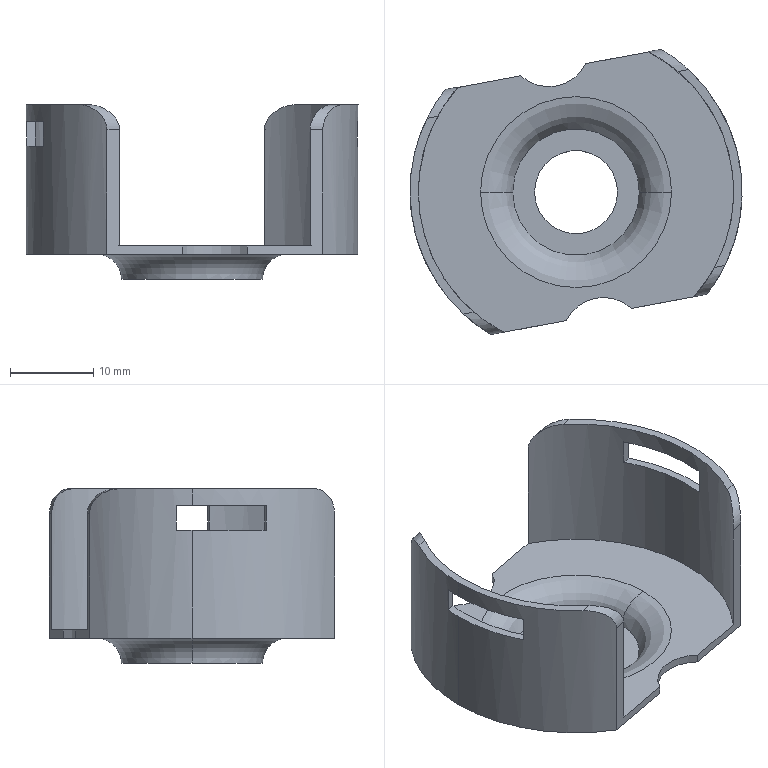Part | SolidWorks | features Cut 4, Fillet 2, Extrusion 1, ICE 1, Shell 1 | 1 solid | 36 faces | box 40 x 34.338 x 21 mm | volume 2143 mm3 | plane 18 | cylinder 14 | torus 4 | commonest cylinder face diameters 6 x4 10 x4 38 x3 40 x3
STEP:
#1=CARTESIAN_POINT('',(-126.531,115.619,0.));
#2=VERTEX_POINT('',#1);
#3=CARTESIAN_POINT('',(-116.531,115.619,0.));
#4=VERTEX_POINT('',#3);
#5=CARTESIAN_POINT('',(-121.531,115.619,0.));
#6=DIRECTION('',(0.,0.,1.));
#7=DIRECTION('',(1.,0.,0.));
#8=AXIS2_PLACEMENT_3D('',#5,#6,#7);
#9=CIRCLE('',#8,5.);
#10=EDGE_CURVE('',#2,#4,#9,.T.);
#11=ORIENTED_EDGE('',*,*,#10,.F.);
#12=CARTESIAN_POINT('',(-126.531,115.619,1.));
#13=VERTEX_POINT('',#12);
#14=CARTESIAN_POINT('',(-126.531,115.619,0.));
#15=DIRECTION('',(0.,0.,1.));
#16=VECTOR('',#15,1000.);
#17=LINE('',#14,#16);
#18=EDGE_CURVE('',#2,#13,#17,.T.);
#19=ORIENTED_EDGE('',*,*,#18,.T.);
#20=CARTESIAN_POINT('',(-116.531,115.619,1.));
#21=VERTEX_POINT('',#20);
#22=CARTESIAN_POINT('',(-121.531,115.619,1.));
#23=DIRECTION('',(0.,0.,-1.));
#24=DIRECTION('',(-1.,0.,0.));
#25=AXIS2_PLACEMENT_3D('',#22,#23,#24);
#26=CIRCLE('',#25,5.);
#27=EDGE_CURVE('',#21,#13,#26,.T.);
#28=ORIENTED_EDGE('',*,*,#27,.F.);
#29=CARTESIAN_POINT('',(-116.531,115.619,0.));
#30=DIRECTION('',(0.,0.,1.));
#31=VECTOR('',#30,1000.);
#32=LINE('',#29,#31);
#33=EDGE_CURVE('',#4,#21,#32,.T.);
#34=ORIENTED_EDGE('',*,*,#33,.F.);
#35=EDGE_LOOP('',(#11,#19,#28,#34));
#36=FACE_OUTER_BOUND('',#35,.T.);
#37=CARTESIAN_POINT('',(-121.531,115.619,0.));
#38=DIRECTION('',(0.,0.,1.));
#39=DIRECTION('',(1.,0.,0.));
#40=AXIS2_PLACEMENT_3D('',#37,#38,#39);
#41=CYLINDRICAL_SURFACE('',#40,5.);
#42=ADVANCED_FACE('',(#36),#41,.F.);
#43=CARTESIAN_POINT('',(-110.031,115.619,4.));
#44=VERTEX_POINT('',#43);
#45=CARTESIAN_POINT('',(-133.031,115.619,4.));
#46=VERTEX_POINT('',#45);
#47=CARTESIAN_POINT('',(-121.531,115.619,4.));
#48=DIRECTION('',(0.,0.,1.));
#49=DIRECTION('',(1.,0.,0.));
#50=AXIS2_PLACEMENT_3D('',#47,#48,#49);
#51=CIRCLE('',#50,11.5);
#52=EDGE_CURVE('',#44,#46,#51,.T.);
#53=ORIENTED_EDGE('',*,*,#52,.T.);
#54=CARTESIAN_POINT('',(-129.158,115.619,1.));
#55=VERTEX_POINT('',#54);
#56=CARTESIAN_POINT('',(-133.031,115.619,0.));
#57=DIRECTION('',(0.,1.,0.));
#58=DIRECTION('',(-1.,0.,0.));
#59=AXIS2_PLACEMENT_3D('',#56,#57,#58);
#60=CIRCLE('',#59,4.);
#61=EDGE_CURVE('',#46,#55,#60,.T.);
#62=ORIENTED_EDGE('',*,*,#61,.T.);
#63=CARTESIAN_POINT('',(-113.904,115.619,1.));
#64=VERTEX_POINT('',#63);
#65=CARTESIAN_POINT('',(-121.531,115.619,1.));
#66=DIRECTION('',(0.,0.,-1.));
#67=DIRECTION('',(1.,0.,0.));
#68=AXIS2_PLACEMENT_3D('',#65,#66,#67);
#69=CIRCLE('',#68,7.627);
#70=EDGE_CURVE('',#55,#64,#69,.T.);
#71=ORIENTED_EDGE('',*,*,#70,.T.);
#72=CARTESIAN_POINT('',(-110.031,115.619,0.));
#73=DIRECTION('',(0.,-1.,0.));
#74=DIRECTION('',(0.,0.,-1.));
#75=AXIS2_PLACEMENT_3D('',#72,#73,#74);
#76=CIRCLE('',#75,4.);
#77=EDGE_CURVE('',#44,#64,#76,.T.);
#78=ORIENTED_EDGE('',*,*,#77,.F.);
#79=EDGE_LOOP('',(#53,#62,#71,#78));
#80=FACE_OUTER_BOUND('',#79,.T.);
#81=CARTESIAN_POINT('',(-121.531,115.619,0.));
#82=DIRECTION('',(0.,0.,1.));
#83=DIRECTION('',(1.,0.,0.));
#84=AXIS2_PLACEMENT_3D('',#81,#82,#83);
#85=TOROIDAL_SURFACE('',#84,11.5,4.);
#86=ADVANCED_FACE('',(#80),#85,.T.);
#87=CARTESIAN_POINT('',(-133.031,115.619,3.));
#88=VERTEX_POINT('',#87);
#89=CARTESIAN_POINT('',(-110.031,115.619,3.));
#90=VERTEX_POINT('',#89);
#91=CARTESIAN_POINT('',(-121.531,115.619,3.));
#92=DIRECTION('',(0.,0.,1.));
#93=DIRECTION('',(1.,0.,0.));
#94=AXIS2_PLACEMENT_3D('',#91,#92,#93);
#95=CIRCLE('',#94,11.5);
#96=EDGE_CURVE('',#88,#90,#95,.T.);
#97=ORIENTED_EDGE('',*,*,#96,.F.);
#98=CARTESIAN_POINT('',(-130.031,115.619,0.));
#99=VERTEX_POINT('',#98);
#100=CARTESIAN_POINT('',(-133.031,115.619,0.));
#101=DIRECTION('',(0.,1.,0.));
#102=DIRECTION('',(-1.,0.,0.));
#103=AXIS2_PLACEMENT_3D('',#100,#101,#102);
#104=CIRCLE('',#103,3.);
#105=EDGE_CURVE('',#88,#99,#104,.T.);
#106=ORIENTED_EDGE('',*,*,#105,.T.);
#107=CARTESIAN_POINT('',(-113.031,115.619,0.));
#108=VERTEX_POINT('',#107);
#109=CARTESIAN_POINT('',(-121.531,115.619,0.));
#110=DIRECTION('',(0.,0.,-1.));
#111=DIRECTION('',(-1.,0.,0.));
#112=AXIS2_PLACEMENT_3D('',#109,#110,#111);
#113=CIRCLE('',#112,8.5);
#114=EDGE_CURVE('',#108,#99,#113,.T.);
#115=ORIENTED_EDGE('',*,*,#114,.F.);
#116=CARTESIAN_POINT('',(-110.031,115.619,0.));
#117=DIRECTION('',(0.,-1.,0.));
#118=DIRECTION('',(0.,0.,-1.));
#119=AXIS2_PLACEMENT_3D('',#116,#117,#118);
#120=CIRCLE('',#119,3.);
#121=EDGE_CURVE('',#90,#108,#120,.T.);
#122=ORIENTED_EDGE('',*,*,#121,.F.);
#123=EDGE_LOOP('',(#97,#106,#115,#122));
#124=FACE_OUTER_BOUND('',#123,.T.);
#125=CARTESIAN_POINT('',(-121.531,115.619,0.));
#126=DIRECTION('',(0.,0.,1.));
#127=DIRECTION('',(1.,0.,0.));
#128=AXIS2_PLACEMENT_3D('',#125,#126,#127);
#129=TOROIDAL_SURFACE('',#128,11.5,3.);
#130=ADVANCED_FACE('',(#124),#129,.F.);
#131=CARTESIAN_POINT('',(-138.211,124.718,21.));
#132=VERTEX_POINT('',#131);
#133=CARTESIAN_POINT('',(-140.531,115.619,21.));
#134=VERTEX_POINT('',#133);
#135=CARTESIAN_POINT('',(-121.531,115.619,21.));
#136=DIRECTION('',(0.,0.,1.));
#137=DIRECTION('',(1.,0.,0.));
#138=AXIS2_PLACEMENT_3D('',#135,#136,#137);
#139=CIRCLE('',#138,19.);
#140=EDGE_CURVE('',#132,#134,#139,.T.);
#141=ORIENTED_EDGE('',*,*,#140,.T.);
#142=CARTESIAN_POINT('',(-140.531,115.619,19.));
#143=VERTEX_POINT('',#142);
#144=CARTESIAN_POINT('',(-140.531,115.619,21.));
#145=DIRECTION('',(0.,0.,-1.));
#146=VECTOR('',#145,1000.);
#147=LINE('',#144,#146);
#148=EDGE_CURVE('',#134,#143,#147,.T.);
#149=ORIENTED_EDGE('',*,*,#148,.T.);
#150=CARTESIAN_POINT('',(-140.417,117.695,19.));
#151=VERTEX_POINT('',#150);
#152=CARTESIAN_POINT('',(-121.531,115.619,19.));
#153=DIRECTION('',(0.,0.,1.));
#154=DIRECTION('',(1.,0.,0.));
#155=AXIS2_PLACEMENT_3D('',#152,#153,#154);
#156=CIRCLE('',#155,19.);
#157=EDGE_CURVE('',#151,#143,#156,.T.);
#158=ORIENTED_EDGE('',*,*,#157,.F.);
#159=CARTESIAN_POINT('',(-140.417,117.695,16.));
#160=VERTEX_POINT('',#159);
#161=CARTESIAN_POINT('',(-140.417,117.695,21.));
#162=DIRECTION('',(0.,0.,1.));
#163=VECTOR('',#162,1000.);
#164=LINE('',#161,#163);
#165=EDGE_CURVE('',#160,#151,#164,.T.);
#166=ORIENTED_EDGE('',*,*,#165,.F.);
#167=CARTESIAN_POINT('',(-140.531,115.619,16.));
#168=VERTEX_POINT('',#167);
#169=CARTESIAN_POINT('',(-121.531,115.619,16.));
#170=DIRECTION('',(0.,0.,-1.));
#171=DIRECTION('',(-1.,0.,0.));
#172=AXIS2_PLACEMENT_3D('',#169,#170,#171);
#173=CIRCLE('',#172,19.);
#174=EDGE_CURVE('',#168,#160,#173,.T.);
#175=ORIENTED_EDGE('',*,*,#174,.F.);
#176=CARTESIAN_POINT('',(-140.531,115.619,4.));
#177=VERTEX_POINT('',#176);
#178=CARTESIAN_POINT('',(-140.531,115.619,21.));
#179=DIRECTION('',(0.,0.,-1.));
#180=VECTOR('',#179,1000.);
#181=LINE('',#178,#180);
#182=EDGE_CURVE('',#168,#177,#181,.T.);
#183=ORIENTED_EDGE('',*,*,#182,.T.);
#184=CARTESIAN_POINT('',(-135.743,128.229,4.));
#185=VERTEX_POINT('',#184);
#186=CARTESIAN_POINT('',(-121.531,115.619,4.));
#187=DIRECTION('',(0.,0.,1.));
#188=DIRECTION('',(1.,0.,0.));
#189=AXIS2_PLACEMENT_3D('',#186,#187,#188);
#190=CIRCLE('',#189,19.);
#191=EDGE_CURVE('',#185,#177,#190,.T.);
#192=ORIENTED_EDGE('',*,*,#191,.F.);
#193=CARTESIAN_POINT('',(-135.743,128.229,18.));
#194=VERTEX_POINT('',#193);
#195=CARTESIAN_POINT('',(-135.743,128.229,21.));
#196=DIRECTION('',(0.,0.,-1.));
#197=VECTOR('',#196,1000.);
#198=LINE('',#195,#197);
#199=EDGE_CURVE('',#194,#185,#198,.T.);
#200=ORIENTED_EDGE('',*,*,#199,.F.);
#201=CARTESIAN_POINT('',(-135.743,128.229,18.));
#202=CARTESIAN_POINT('',(-135.743,128.229,18.243));
#203=CARTESIAN_POINT('',(-135.775,128.194,18.475));
#204=CARTESIAN_POINT('',(-135.889,128.063,18.925));
#205=CARTESIAN_POINT('',(-135.97,127.97,19.132));
#206=CARTESIAN_POINT('',(-136.16,127.745,19.512));
#207=CARTESIAN_POINT('',(-136.267,127.614,19.683));
#208=CARTESIAN_POINT('',(-136.494,127.33,19.99));
#209=CARTESIAN_POINT('',(-136.615,127.174,20.128));
#210=CARTESIAN_POINT('',(-136.984,126.681,20.496));
#211=CARTESIAN_POINT('',(-137.236,126.323,20.678));
#212=CARTESIAN_POINT('',(-137.612,125.741,20.869));
#213=CARTESIAN_POINT('',(-137.736,125.542,20.917));
#214=CARTESIAN_POINT('',(-137.978,125.136,20.983));
#215=CARTESIAN_POINT('',(-138.096,124.929,21.));
#216=CARTESIAN_POINT('',(-138.211,124.718,21.));
#217=B_SPLINE_CURVE_WITH_KNOTS('',3,(#201,#202,#203,#204,#205,#206,#207,#208,#209,#210,#211,#212,#213,#214,#215,#216),.UNSPECIFIED.,.F.,.F.,(4,2,2,2,2,2,2,4),(0.,0.0007129,0.001426,0.002139,0.002852,0.004277,0.00499,0.005703),.UNSPECIFIED.);
#218=EDGE_CURVE('',#194,#132,#217,.T.);
#219=ORIENTED_EDGE('',*,*,#218,.T.);
#220=EDGE_LOOP('',(#141,#149,#158,#166,#175,#183,#192,#200,#219));
#221=FACE_OUTER_BOUND('',#220,.T.);
#222=CARTESIAN_POINT('',(-121.531,115.619,21.));
#223=DIRECTION('',(0.,0.,-1.));
#224=DIRECTION('',(-1.,0.,0.));
#225=AXIS2_PLACEMENT_3D('',#222,#223,#224);
#226=CYLINDRICAL_SURFACE('',#225,19.);
#227=ADVANCED_FACE('',(#221),#226,.F.);
#228=CARTESIAN_POINT('',(-141.531,115.619,21.));
#229=VERTEX_POINT('',#228);
#230=CARTESIAN_POINT('',(-135.063,100.892,21.));
#231=VERTEX_POINT('',#230);
#232=CARTESIAN_POINT('',(-121.531,115.619,21.));
#233=DIRECTION('',(0.,0.,1.));
#234=DIRECTION('',(1.,0.,0.));
#235=AXIS2_PLACEMENT_3D('',#232,#233,#234);
#236=CIRCLE('',#235,20.);
#237=EDGE_CURVE('',#229,#231,#236,.T.);
#238=ORIENTED_EDGE('',*,*,#237,.F.);
#239=CARTESIAN_POINT('',(-141.531,115.619,19.));
#240=VERTEX_POINT('',#239);
#241=CARTESIAN_POINT('',(-141.531,115.619,21.));
#242=DIRECTION('',(0.,0.,-1.));
#243=VECTOR('',#242,1000.);
#244=LINE('',#241,#243);
#245=EDGE_CURVE('',#229,#240,#244,.T.);
#246=ORIENTED_EDGE('',*,*,#245,.T.);
#247=CARTESIAN_POINT('',(-139.427,106.69,19.));
#248=VERTEX_POINT('',#247);
#249=CARTESIAN_POINT('',(-121.531,115.619,19.));
#250=DIRECTION('',(0.,0.,1.));
#251=DIRECTION('',(1.,0.,0.));
#252=AXIS2_PLACEMENT_3D('',#249,#250,#251);
#253=CIRCLE('',#252,20.);
#254=EDGE_CURVE('',#240,#248,#253,.T.);
#255=ORIENTED_EDGE('',*,*,#254,.T.);
#256=CARTESIAN_POINT('',(-139.427,106.69,16.));
#257=VERTEX_POINT('',#256);
#258=CARTESIAN_POINT('',(-139.427,106.69,21.));
#259=DIRECTION('',(0.,0.,-1.));
#260=VECTOR('',#259,1000.);
#261=LINE('',#258,#260);
#262=EDGE_CURVE('',#248,#257,#261,.T.);
#263=ORIENTED_EDGE('',*,*,#262,.T.);
#264=CARTESIAN_POINT('',(-141.531,115.619,16.));
#265=VERTEX_POINT('',#264);
#266=CARTESIAN_POINT('',(-121.531,115.619,16.));
#267=DIRECTION('',(0.,0.,-1.));
#268=DIRECTION('',(-1.,0.,0.));
#269=AXIS2_PLACEMENT_3D('',#266,#267,#268);
#270=CIRCLE('',#269,20.);
#271=EDGE_CURVE('',#257,#265,#270,.T.);
#272=ORIENTED_EDGE('',*,*,#271,.T.);
#273=CARTESIAN_POINT('',(-141.531,115.619,3.));
#274=VERTEX_POINT('',#273);
#275=CARTESIAN_POINT('',(-141.531,115.619,21.));
#276=DIRECTION('',(0.,0.,-1.));
#277=VECTOR('',#276,1000.);
#278=LINE('',#275,#277);
#279=EDGE_CURVE('',#265,#274,#278,.T.);
#280=ORIENTED_EDGE('',*,*,#279,.T.);
#281=CARTESIAN_POINT('',(-131.789,98.45,3.));
#282=VERTEX_POINT('',#281);
#283=CARTESIAN_POINT('',(-121.531,115.619,3.));
#284=DIRECTION('',(0.,0.,1.));
#285=DIRECTION('',(1.,0.,0.));
#286=AXIS2_PLACEMENT_3D('',#283,#284,#285);
#287=CIRCLE('',#286,20.);
#288=EDGE_CURVE('',#274,#282,#287,.T.);
#289=ORIENTED_EDGE('',*,*,#288,.T.);
#290=CARTESIAN_POINT('',(-131.789,98.45,18.));
#291=VERTEX_POINT('',#290);
#292=CARTESIAN_POINT('',(-131.789,98.45,21.));
#293=DIRECTION('',(0.,0.,1.));
#294=VECTOR('',#293,1000.);
#295=LINE('',#292,#294);
#296=EDGE_CURVE('',#282,#291,#295,.T.);
#297=ORIENTED_EDGE('',*,*,#296,.T.);
#298=CARTESIAN_POINT('',(-131.789,98.45,18.));
#299=CARTESIAN_POINT('',(-131.789,98.45,18.235));
#300=CARTESIAN_POINT('',(-131.824,98.471,18.462));
#301=CARTESIAN_POINT('',(-131.956,98.551,18.902));
#302=CARTESIAN_POINT('',(-132.051,98.609,19.109));
#303=CARTESIAN_POINT('',(-132.279,98.752,19.488));
#304=CARTESIAN_POINT('',(-132.412,98.837,19.662));
#305=CARTESIAN_POINT('',(-132.697,99.025,19.973));
#306=CARTESIAN_POINT('',(-132.85,99.129,20.113));
#307=CARTESIAN_POINT('',(-133.333,99.468,20.489));
#308=CARTESIAN_POINT('',(-133.672,99.719,20.674));
#309=CARTESIAN_POINT('',(-134.194,100.137,20.867));
#310=CARTESIAN_POINT('',(-134.37,100.282,20.917));
#311=CARTESIAN_POINT('',(-134.718,100.58,20.983));
#312=CARTESIAN_POINT('',(-134.891,100.734,21.));
#313=CARTESIAN_POINT('',(-135.063,100.892,21.));
#314=B_SPLINE_CURVE_WITH_KNOTS('',3,(#298,#299,#300,#301,#302,#303,#304,#305,#306,#307,#308,#309,#310,#311,#312,#313),.UNSPECIFIED.,.F.,.F.,(4,2,2,2,2,2,2,4),(0.,0.0006922,0.001384,0.002077,0.002769,0.004153,0.004846,0.005538),.UNSPECIFIED.);
#315=EDGE_CURVE('',#291,#231,#314,.T.);
#316=ORIENTED_EDGE('',*,*,#315,.T.);
#317=EDGE_LOOP('',(#238,#246,#255,#263,#272,#280,#289,#297,#316));
#318=FACE_OUTER_BOUND('',#317,.T.);
#319=CARTESIAN_POINT('',(-121.531,115.619,21.));
#320=DIRECTION('',(0.,0.,-1.));
#321=DIRECTION('',(-1.,0.,0.));
#322=AXIS2_PLACEMENT_3D('',#319,#320,#321);
#323=CYLINDRICAL_SURFACE('',#322,20.);
#324=ADVANCED_FACE('',(#318),#323,.T.);
#325=CARTESIAN_POINT('',(-122.716,100.14,3.));
#326=VERTEX_POINT('',#325);
#327=CARTESIAN_POINT('',(-63.278,111.213,3.));
#328=DIRECTION('',(0.9831,0.1831,0.));
#329=VECTOR('',#328,1000.);
#330=LINE('',#327,#329);
#331=EDGE_CURVE('',#282,#326,#330,.T.);
#332=ORIENTED_EDGE('',*,*,#331,.T.);
#333=CARTESIAN_POINT('',(-122.716,100.14,4.));
#334=VERTEX_POINT('',#333);
#335=CARTESIAN_POINT('',(-122.716,100.14,-11.142));
#336=DIRECTION('',(0.,0.,1.));
#337=VECTOR('',#336,1000.);
#338=LINE('',#335,#337);
#339=EDGE_CURVE('',#326,#334,#338,.T.);
#340=ORIENTED_EDGE('',*,*,#339,.T.);
#341=CARTESIAN_POINT('',(-130.249,98.737,4.));
#342=VERTEX_POINT('',#341);
#343=CARTESIAN_POINT('',(-118.784,100.873,4.));
#344=DIRECTION('',(-0.9831,-0.1831,0.));
#345=VECTOR('',#344,1000.);
#346=LINE('',#343,#345);
#347=EDGE_CURVE('',#334,#342,#346,.T.);
#348=ORIENTED_EDGE('',*,*,#347,.T.);
#349=CARTESIAN_POINT('',(-130.249,98.737,18.));
#350=VERTEX_POINT('',#349);
#351=CARTESIAN_POINT('',(-130.249,98.737,21.));
#352=DIRECTION('',(0.,0.,1.));
#353=VECTOR('',#352,1000.);
#354=LINE('',#351,#353);
#355=EDGE_CURVE('',#342,#350,#354,.T.);
#356=ORIENTED_EDGE('',*,*,#355,.T.);
#357=CARTESIAN_POINT('',(-131.789,98.45,18.));
#358=DIRECTION('',(-0.9831,-0.1831,0.));
#359=VECTOR('',#358,1000.);
#360=LINE('',#357,#359);
#361=EDGE_CURVE('',#350,#291,#360,.T.);
#362=ORIENTED_EDGE('',*,*,#361,.T.);
#363=ORIENTED_EDGE('',*,*,#296,.F.);
#364=EDGE_LOOP('',(#332,#340,#348,#356,#362,#363));
#365=FACE_OUTER_BOUND('',#364,.T.);
#366=CARTESIAN_POINT('',(-63.278,111.213,-77.678));
#367=DIRECTION('',(-0.1831,0.9831,0.));
#368=DIRECTION('',(-0.9831,-0.1831,0.));
#369=AXIS2_PLACEMENT_3D('',#366,#367,#368);
#370=PLANE('',#369);
#371=ADVANCED_FACE('',(#365),#370,.F.);
#372=CARTESIAN_POINT('',(-111.273,132.788,3.));
#373=VERTEX_POINT('',#372);
#374=CARTESIAN_POINT('',(-120.346,131.098,3.));
#375=VERTEX_POINT('',#374);
#376=CARTESIAN_POINT('',(-106.336,133.708,3.));
#377=DIRECTION('',(-0.9831,-0.1831,0.));
#378=VECTOR('',#377,1000.);
#379=LINE('',#376,#378);
#380=EDGE_CURVE('',#373,#375,#379,.T.);
#381=ORIENTED_EDGE('',*,*,#380,.T.);
#382=CARTESIAN_POINT('',(-120.346,131.098,4.));
#383=VERTEX_POINT('',#382);
#384=CARTESIAN_POINT('',(-120.346,131.098,-11.142));
#385=DIRECTION('',(0.,0.,1.));
#386=VECTOR('',#385,1000.);
#387=LINE('',#384,#386);
#388=EDGE_CURVE('',#375,#383,#387,.T.);
#389=ORIENTED_EDGE('',*,*,#388,.T.);
#390=CARTESIAN_POINT('',(-112.814,132.501,4.));
#391=VERTEX_POINT('',#390);
#392=CARTESIAN_POINT('',(-124.278,130.365,4.));
#393=DIRECTION('',(0.9831,0.1831,0.));
#394=VECTOR('',#393,1000.);
#395=LINE('',#392,#394);
#396=EDGE_CURVE('',#383,#391,#395,.T.);
#397=ORIENTED_EDGE('',*,*,#396,.T.);
#398=CARTESIAN_POINT('',(-112.814,132.501,18.));
#399=VERTEX_POINT('',#398);
#400=CARTESIAN_POINT('',(-112.814,132.501,21.));
#401=DIRECTION('',(0.,0.,1.));
#402=VECTOR('',#401,1000.);
#403=LINE('',#400,#402);
#404=EDGE_CURVE('',#391,#399,#403,.T.);
#405=ORIENTED_EDGE('',*,*,#404,.T.);
#406=CARTESIAN_POINT('',(-111.273,132.788,18.));
#407=VERTEX_POINT('',#406);
#408=CARTESIAN_POINT('',(-111.273,132.788,18.));
#409=DIRECTION('',(0.9831,0.1831,0.));
#410=VECTOR('',#409,1000.);
#411=LINE('',#408,#410);
#412=EDGE_CURVE('',#399,#407,#411,.T.);
#413=ORIENTED_EDGE('',*,*,#412,.T.);
#414=CARTESIAN_POINT('',(-111.273,132.788,21.));
#415=DIRECTION('',(0.,0.,1.));
#416=VECTOR('',#415,1000.);
#417=LINE('',#414,#416);
#418=EDGE_CURVE('',#373,#407,#417,.T.);
#419=ORIENTED_EDGE('',*,*,#418,.F.);
#420=EDGE_LOOP('',(#381,#389,#397,#405,#413,#419));
#421=FACE_OUTER_BOUND('',#420,.T.);
#422=CARTESIAN_POINT('',(-106.336,133.708,-77.678));
#423=DIRECTION('',(0.1831,-0.9831,0.));
#424=DIRECTION('',(0.9831,0.1831,0.));
#425=AXIS2_PLACEMENT_3D('',#422,#423,#424);
#426=PLANE('',#425);
#427=ADVANCED_FACE('',(#421),#426,.F.);
#428=ORIENTED_EDGE('',*,*,#245,.F.);
#429=CARTESIAN_POINT('',(-139.458,124.486,21.));
#430=VERTEX_POINT('',#429);
#431=CARTESIAN_POINT('',(-121.531,115.619,21.));
#432=DIRECTION('',(0.,0.,1.));
#433=DIRECTION('',(1.,0.,0.));
#434=AXIS2_PLACEMENT_3D('',#431,#432,#433);
#435=CIRCLE('',#434,20.);
#436=EDGE_CURVE('',#430,#229,#435,.T.);
#437=ORIENTED_EDGE('',*,*,#436,.F.);
#438=CARTESIAN_POINT('',(-137.283,127.942,18.));
#439=VERTEX_POINT('',#438);
#440=CARTESIAN_POINT('',(-139.458,124.486,21.));
#441=CARTESIAN_POINT('',(-139.251,124.904,21.));
#442=CARTESIAN_POINT('',(-139.035,125.305,20.933));
#443=CARTESIAN_POINT('',(-138.697,125.884,20.74));
#444=CARTESIAN_POINT('',(-138.584,126.071,20.66));
#445=CARTESIAN_POINT('',(-138.36,126.428,20.473));
#446=CARTESIAN_POINT('',(-138.249,126.598,20.365));
#447=CARTESIAN_POINT('',(-138.032,126.921,20.117));
#448=CARTESIAN_POINT('',(-137.925,127.076,19.976));
#449=CARTESIAN_POINT('',(-137.726,127.355,19.664));
#450=CARTESIAN_POINT('',(-137.634,127.481,19.493));
#451=CARTESIAN_POINT('',(-137.472,127.699,19.111));
#452=CARTESIAN_POINT('',(-137.405,127.786,18.907));
#453=CARTESIAN_POINT('',(-137.333,127.878,18.577));
#454=CARTESIAN_POINT('',(-137.315,127.902,18.463));
#455=CARTESIAN_POINT('',(-137.29,127.934,18.234));
#456=CARTESIAN_POINT('',(-137.283,127.942,18.118));
#457=CARTESIAN_POINT('',(-137.283,127.942,18.));
#458=B_SPLINE_CURVE_WITH_KNOTS('',3,(#440,#441,#442,#443,#444,#445,#446,#447,#448,#449,#450,#451,#452,#453,#454,#455,#456,#457),.UNSPECIFIED.,.F.,.F.,(4,2,2,2,2,2,2,2,4),(0.,0.001383,0.002074,0.002765,0.003456,0.004148,0.004839,0.005185,0.00553),.UNSPECIFIED.);
#459=EDGE_CURVE('',#430,#439,#458,.T.);
#460=ORIENTED_EDGE('',*,*,#459,.T.);
#461=CARTESIAN_POINT('',(-137.283,127.942,3.));
#462=VERTEX_POINT('',#461);
#463=CARTESIAN_POINT('',(-137.283,127.942,21.));
#464=DIRECTION('',(0.,0.,-1.));
#465=VECTOR('',#464,1000.);
#466=LINE('',#463,#465);
#467=EDGE_CURVE('',#439,#462,#466,.T.);
#468=ORIENTED_EDGE('',*,*,#467,.T.);
#469=CARTESIAN_POINT('',(-121.531,115.619,3.));
#470=DIRECTION('',(0.,0.,1.));
#471=DIRECTION('',(1.,0.,0.));
#472=AXIS2_PLACEMENT_3D('',#469,#470,#471);
#473=CIRCLE('',#472,20.);
#474=EDGE_CURVE('',#462,#274,#473,.T.);
#475=ORIENTED_EDGE('',*,*,#474,.T.);
#476=ORIENTED_EDGE('',*,*,#279,.F.);
#477=CARTESIAN_POINT('',(-141.442,117.504,16.));
#478=VERTEX_POINT('',#477);
#479=CARTESIAN_POINT('',(-121.531,115.619,16.));
#480=DIRECTION('',(0.,0.,-1.));
#481=DIRECTION('',(-1.,0.,0.));
#482=AXIS2_PLACEMENT_3D('',#479,#480,#481);
#483=CIRCLE('',#482,20.);
#484=EDGE_CURVE('',#265,#478,#483,.T.);
#485=ORIENTED_EDGE('',*,*,#484,.T.);
#486=CARTESIAN_POINT('',(-141.442,117.504,19.));
#487=VERTEX_POINT('',#486);
#488=CARTESIAN_POINT('',(-141.442,117.504,21.));
#489=DIRECTION('',(0.,0.,1.));
#490=VECTOR('',#489,1000.);
#491=LINE('',#488,#490);
#492=EDGE_CURVE('',#478,#487,#491,.T.);
#493=ORIENTED_EDGE('',*,*,#492,.T.);
#494=CARTESIAN_POINT('',(-121.531,115.619,19.));
#495=DIRECTION('',(0.,0.,1.));
#496=DIRECTION('',(1.,0.,0.));
#497=AXIS2_PLACEMENT_3D('',#494,#495,#496);
#498=CIRCLE('',#497,20.);
#499=EDGE_CURVE('',#487,#240,#498,.T.);
#500=ORIENTED_EDGE('',*,*,#499,.T.);
#501=EDGE_LOOP('',(#428,#437,#460,#468,#475,#476,#485,#493,#500));
#502=FACE_OUTER_BOUND('',#501,.T.);
#503=CARTESIAN_POINT('',(-121.531,115.619,21.));
#504=DIRECTION('',(0.,0.,-1.));
#505=DIRECTION('',(-1.,0.,0.));
#506=AXIS2_PLACEMENT_3D('',#503,#504,#505);
#507=CYLINDRICAL_SURFACE('',#506,20.);
#508=ADVANCED_FACE('',(#502),#507,.T.);
#509=ORIENTED_EDGE('',*,*,#140,.F.);
#510=CARTESIAN_POINT('',(-136.734,124.993,21.));
#511=DIRECTION('',(-0.9831,-0.1831,0.));
#512=VECTOR('',#511,1000.);
#513=LINE('',#510,#512);
#514=EDGE_CURVE('',#132,#430,#513,.T.);
#515=ORIENTED_EDGE('',*,*,#514,.T.);
#516=ORIENTED_EDGE('',*,*,#436,.T.);
#517=ORIENTED_EDGE('',*,*,#237,.T.);
#518=CARTESIAN_POINT('',(-133.815,101.124,21.));
#519=VERTEX_POINT('',#518);
#520=CARTESIAN_POINT('',(-130.798,101.686,21.));
#521=DIRECTION('',(0.9831,0.1831,0.));
#522=VECTOR('',#521,1000.);
#523=LINE('',#520,#522);
#524=EDGE_CURVE('',#231,#519,#523,.T.);
#525=ORIENTED_EDGE('',*,*,#524,.T.);
#526=CARTESIAN_POINT('',(-121.531,115.619,21.));
#527=DIRECTION('',(0.,0.,1.));
#528=DIRECTION('',(1.,0.,0.));
#529=AXIS2_PLACEMENT_3D('',#526,#527,#528);
#530=CIRCLE('',#529,19.);
#531=EDGE_CURVE('',#134,#519,#530,.T.);
#532=ORIENTED_EDGE('',*,*,#531,.F.);
#533=EDGE_LOOP('',(#509,#515,#516,#517,#525,#532));
#534=FACE_OUTER_BOUND('',#533,.T.);
#535=CARTESIAN_POINT('',(-121.531,115.619,21.));
#536=DIRECTION('',(0.,0.,1.));
#537=DIRECTION('',(1.,0.,0.));
#538=AXIS2_PLACEMENT_3D('',#535,#536,#537);
#539=PLANE('',#538);
#540=ADVANCED_FACE('',(#534),#539,.T.);
#541=ORIENTED_EDGE('',*,*,#148,.F.);
#542=ORIENTED_EDGE('',*,*,#531,.T.);
#543=CARTESIAN_POINT('',(-133.815,101.124,21.));
#544=CARTESIAN_POINT('',(-133.448,100.813,21.));
#545=CARTESIAN_POINT('',(-133.078,100.523,20.933));
#546=CARTESIAN_POINT('',(-132.33,99.98,20.679));
#547=CARTESIAN_POINT('',(-131.964,99.735,20.496));
#548=CARTESIAN_POINT('',(-131.445,99.409,20.131));
#549=CARTESIAN_POINT('',(-131.275,99.307,19.992));
#550=CARTESIAN_POINT('',(-130.96,99.123,19.684));
#551=CARTESIAN_POINT('',(-130.813,99.04,19.514));
#552=CARTESIAN_POINT('',(-130.554,98.898,19.133));
#553=CARTESIAN_POINT('',(-130.446,98.84,18.928));
#554=CARTESIAN_POINT('',(-130.291,98.759,18.479));
#555=CARTESIAN_POINT('',(-130.249,98.737,18.242));
#556=CARTESIAN_POINT('',(-130.249,98.737,18.));
#557=B_SPLINE_CURVE_WITH_KNOTS('',3,(#543,#544,#545,#546,#547,#548,#549,#550,#551,#552,#553,#554,#555,#556),.UNSPECIFIED.,.F.,.F.,(4,2,2,2,2,2,4),(0.,0.001426,0.002852,0.003565,0.004278,0.004991,0.005705),.UNSPECIFIED.);
#558=EDGE_CURVE('',#519,#350,#557,.T.);
#559=ORIENTED_EDGE('',*,*,#558,.T.);
#560=ORIENTED_EDGE('',*,*,#355,.F.);
#561=CARTESIAN_POINT('',(-121.531,115.619,4.));
#562=DIRECTION('',(0.,0.,1.));
#563=DIRECTION('',(1.,0.,0.));
#564=AXIS2_PLACEMENT_3D('',#561,#562,#563);
#565=CIRCLE('',#564,19.);
#566=EDGE_CURVE('',#177,#342,#565,.T.);
#567=ORIENTED_EDGE('',*,*,#566,.F.);
#568=ORIENTED_EDGE('',*,*,#182,.F.);
#569=CARTESIAN_POINT('',(-138.403,106.881,16.));
#570=VERTEX_POINT('',#569);
#571=CARTESIAN_POINT('',(-121.531,115.619,16.));
#572=DIRECTION('',(0.,0.,-1.));
#573=DIRECTION('',(-1.,0.,0.));
#574=AXIS2_PLACEMENT_3D('',#571,#572,#573);
#575=CIRCLE('',#574,19.);
#576=EDGE_CURVE('',#570,#168,#575,.T.);
#577=ORIENTED_EDGE('',*,*,#576,.F.);
#578=CARTESIAN_POINT('',(-138.403,106.881,19.));
#579=VERTEX_POINT('',#578);
#580=CARTESIAN_POINT('',(-138.403,106.881,21.));
#581=DIRECTION('',(0.,0.,-1.));
#582=VECTOR('',#581,1000.);
#583=LINE('',#580,#582);
#584=EDGE_CURVE('',#579,#570,#583,.T.);
#585=ORIENTED_EDGE('',*,*,#584,.F.);
#586=CARTESIAN_POINT('',(-121.531,115.619,19.));
#587=DIRECTION('',(0.,0.,1.));
#588=DIRECTION('',(1.,0.,0.));
#589=AXIS2_PLACEMENT_3D('',#586,#587,#588);
#590=CIRCLE('',#589,19.);
#591=EDGE_CURVE('',#143,#579,#590,.T.);
#592=ORIENTED_EDGE('',*,*,#591,.F.);
#593=EDGE_LOOP('',(#541,#542,#559,#560,#567,#568,#577,#585,#592));
#594=FACE_OUTER_BOUND('',#593,.T.);
#595=CARTESIAN_POINT('',(-121.531,115.619,21.));
#596=DIRECTION('',(0.,0.,-1.));
#597=DIRECTION('',(-1.,0.,0.));
#598=AXIS2_PLACEMENT_3D('',#595,#596,#597);
#599=CYLINDRICAL_SURFACE('',#598,19.);
#600=ADVANCED_FACE('',(#594),#599,.F.);
#601=CARTESIAN_POINT('',(-103.635,124.548,16.));
#602=VERTEX_POINT('',#601);
#603=CARTESIAN_POINT('',(-101.62,113.734,16.));
#604=VERTEX_POINT('',#603);
#605=CARTESIAN_POINT('',(-121.531,115.619,16.));
#606=DIRECTION('',(0.,0.,-1.));
#607=DIRECTION('',(-1.,0.,0.));
#608=AXIS2_PLACEMENT_3D('',#605,#606,#607);
#609=CIRCLE('',#608,20.);
#610=EDGE_CURVE('',#602,#604,#609,.T.);
#611=ORIENTED_EDGE('',*,*,#610,.T.);
#612=CARTESIAN_POINT('',(-101.62,113.734,19.));
#613=VERTEX_POINT('',#612);
#614=CARTESIAN_POINT('',(-101.62,113.734,21.));
#615=DIRECTION('',(0.,0.,1.));
#616=VECTOR('',#615,1000.);
#617=LINE('',#614,#616);
#618=EDGE_CURVE('',#604,#613,#617,.T.);
#619=ORIENTED_EDGE('',*,*,#618,.T.);
#620=CARTESIAN_POINT('',(-103.635,124.548,19.));
#621=VERTEX_POINT('',#620);
#622=CARTESIAN_POINT('',(-121.531,115.619,19.));
#623=DIRECTION('',(0.,0.,1.));
#624=DIRECTION('',(1.,0.,0.));
#625=AXIS2_PLACEMENT_3D('',#622,#623,#624);
#626=CIRCLE('',#625,20.);
#627=EDGE_CURVE('',#613,#621,#626,.T.);
#628=ORIENTED_EDGE('',*,*,#627,.T.);
#629=CARTESIAN_POINT('',(-103.635,124.548,21.));
#630=DIRECTION('',(0.,0.,-1.));
#631=VECTOR('',#630,1000.);
#632=LINE('',#629,#631);
#633=EDGE_CURVE('',#621,#602,#632,.T.);
#634=ORIENTED_EDGE('',*,*,#633,.T.);
#635=EDGE_LOOP('',(#611,#619,#628,#634));
#636=FACE_BOUND('',#635,.T.);
#637=ORIENTED_EDGE('',*,*,#418,.T.);
#638=CARTESIAN_POINT('',(-108.,130.346,21.));
#639=VERTEX_POINT('',#638);
#640=CARTESIAN_POINT('',(-111.273,132.788,18.));
#641=CARTESIAN_POINT('',(-111.273,132.788,18.235));
#642=CARTESIAN_POINT('',(-111.238,132.767,18.462));
#643=CARTESIAN_POINT('',(-111.106,132.687,18.902));
#644=CARTESIAN_POINT('',(-111.011,132.629,19.109));
#645=CARTESIAN_POINT('',(-110.783,132.486,19.488));
#646=CARTESIAN_POINT('',(-110.65,132.401,19.662));
#647=CARTESIAN_POINT('',(-110.365,132.213,19.973));
#648=CARTESIAN_POINT('',(-110.212,132.109,20.113));
#649=CARTESIAN_POINT('',(-109.729,131.77,20.489));
#650=CARTESIAN_POINT('',(-109.391,131.519,20.674));
#651=CARTESIAN_POINT('',(-108.868,131.101,20.867));
#652=CARTESIAN_POINT('',(-108.692,130.956,20.917));
#653=CARTESIAN_POINT('',(-108.344,130.658,20.983));
#654=CARTESIAN_POINT('',(-108.171,130.504,21.));
#655=CARTESIAN_POINT('',(-108.,130.346,21.));
#656=B_SPLINE_CURVE_WITH_KNOTS('',3,(#640,#641,#642,#643,#644,#645,#646,#647,#648,#649,#650,#651,#652,#653,#654,#655),.UNSPECIFIED.,.F.,.F.,(4,2,2,2,2,2,2,4),(0.,0.0006922,0.001384,0.002077,0.002769,0.004153,0.004846,0.005538),.UNSPECIFIED.);
#657=EDGE_CURVE('',#407,#639,#656,.T.);
#658=ORIENTED_EDGE('',*,*,#657,.T.);
#659=CARTESIAN_POINT('',(-103.604,106.752,21.));
#660=VERTEX_POINT('',#659);
#661=CARTESIAN_POINT('',(-121.531,115.619,21.));
#662=DIRECTION('',(0.,0.,1.));
#663=DIRECTION('',(1.,0.,0.));
#664=AXIS2_PLACEMENT_3D('',#661,#662,#663);
#665=CIRCLE('',#664,20.);
#666=EDGE_CURVE('',#660,#639,#665,.T.);
#667=ORIENTED_EDGE('',*,*,#666,.F.);
#668=CARTESIAN_POINT('',(-105.779,103.296,18.));
#669=VERTEX_POINT('',#668);
#670=CARTESIAN_POINT('',(-103.604,106.752,21.));
#671=CARTESIAN_POINT('',(-103.811,106.334,21.));
#672=CARTESIAN_POINT('',(-104.028,105.933,20.933));
#673=CARTESIAN_POINT('',(-104.365,105.354,20.74));
#674=CARTESIAN_POINT('',(-104.479,105.167,20.66));
#675=CARTESIAN_POINT('',(-104.702,104.81,20.473));
#676=CARTESIAN_POINT('',(-104.813,104.64,20.365));
#677=CARTESIAN_POINT('',(-105.03,104.317,20.117));
#678=CARTESIAN_POINT('',(-105.137,104.162,19.976));
#679=CARTESIAN_POINT('',(-105.336,103.883,19.664));
#680=CARTESIAN_POINT('',(-105.428,103.757,19.493));
#681=CARTESIAN_POINT('',(-105.591,103.539,19.111));
#682=CARTESIAN_POINT('',(-105.658,103.452,18.907));
#683=CARTESIAN_POINT('',(-105.729,103.36,18.577));
#684=CARTESIAN_POINT('',(-105.748,103.336,18.463));
#685=CARTESIAN_POINT('',(-105.773,103.304,18.234));
#686=CARTESIAN_POINT('',(-105.779,103.296,18.118));
#687=CARTESIAN_POINT('',(-105.779,103.296,18.));
#688=B_SPLINE_CURVE_WITH_KNOTS('',3,(#670,#671,#672,#673,#674,#675,#676,#677,#678,#679,#680,#681,#682,#683,#684,#685,#686,#687),.UNSPECIFIED.,.F.,.F.,(4,2,2,2,2,2,2,2,4),(0.,0.001383,0.002074,0.002765,0.003456,0.004148,0.004839,0.005185,0.00553),.UNSPECIFIED.);
#689=EDGE_CURVE('',#660,#669,#688,.T.);
#690=ORIENTED_EDGE('',*,*,#689,.T.);
#691=CARTESIAN_POINT('',(-105.779,103.296,3.));
#692=VERTEX_POINT('',#691);
#693=CARTESIAN_POINT('',(-105.779,103.296,21.));
#694=DIRECTION('',(0.,0.,-1.));
#695=VECTOR('',#694,1000.);
#696=LINE('',#693,#695);
#697=EDGE_CURVE('',#669,#692,#696,.T.);
#698=ORIENTED_EDGE('',*,*,#697,.T.);
#699=CARTESIAN_POINT('',(-121.531,115.619,3.));
#700=DIRECTION('',(0.,0.,1.));
#701=DIRECTION('',(1.,0.,0.));
#702=AXIS2_PLACEMENT_3D('',#699,#700,#701);
#703=CIRCLE('',#702,20.);
#704=EDGE_CURVE('',#692,#373,#703,.T.);
#705=ORIENTED_EDGE('',*,*,#704,.T.);
#706=EDGE_LOOP('',(#637,#658,#667,#690,#698,#705));
#707=FACE_OUTER_BOUND('',#706,.T.);
#708=CARTESIAN_POINT('',(-121.531,115.619,21.));
#709=DIRECTION('',(0.,0.,-1.));
#710=DIRECTION('',(-1.,0.,0.));
#711=AXIS2_PLACEMENT_3D('',#708,#709,#710);
#712=CYLINDRICAL_SURFACE('',#711,20.);
#713=ADVANCED_FACE('',(#636,#707),#712,.T.);
#714=ORIENTED_EDGE('',*,*,#666,.T.);
#715=CARTESIAN_POINT('',(-109.247,130.114,21.));
#716=VERTEX_POINT('',#715);
#717=CARTESIAN_POINT('',(-112.264,129.552,21.));
#718=DIRECTION('',(-0.9831,-0.1831,0.));
#719=VECTOR('',#718,1000.);
#720=LINE('',#717,#719);
#721=EDGE_CURVE('',#639,#716,#720,.T.);
#722=ORIENTED_EDGE('',*,*,#721,.T.);
#723=CARTESIAN_POINT('',(-104.852,106.52,21.));
#724=VERTEX_POINT('',#723);
#725=CARTESIAN_POINT('',(-121.531,115.619,21.));
#726=DIRECTION('',(0.,0.,1.));
#727=DIRECTION('',(1.,0.,0.));
#728=AXIS2_PLACEMENT_3D('',#725,#726,#727);
#729=CIRCLE('',#728,19.);
#730=EDGE_CURVE('',#724,#716,#729,.T.);
#731=ORIENTED_EDGE('',*,*,#730,.F.);
#732=CARTESIAN_POINT('',(-106.328,106.245,21.));
#733=DIRECTION('',(0.9831,0.1831,0.));
#734=VECTOR('',#733,1000.);
#735=LINE('',#732,#734);
#736=EDGE_CURVE('',#724,#660,#735,.T.);
#737=ORIENTED_EDGE('',*,*,#736,.T.);
#738=EDGE_LOOP('',(#714,#722,#731,#737));
#739=FACE_OUTER_BOUND('',#738,.T.);
#740=CARTESIAN_POINT('',(-121.531,115.619,21.));
#741=DIRECTION('',(0.,0.,1.));
#742=DIRECTION('',(1.,0.,0.));
#743=AXIS2_PLACEMENT_3D('',#740,#741,#742);
#744=PLANE('',#743);
#745=ADVANCED_FACE('',(#739),#744,.T.);
#746=CARTESIAN_POINT('',(-121.531,115.619,3.));
#747=DIRECTION('',(0.,0.,1.));
#748=DIRECTION('',(1.,0.,0.));
#749=AXIS2_PLACEMENT_3D('',#746,#747,#748);
#750=CIRCLE('',#749,11.5);
#751=EDGE_CURVE('',#90,#88,#750,.T.);
#752=ORIENTED_EDGE('',*,*,#751,.T.);
#753=ORIENTED_EDGE('',*,*,#96,.T.);
#754=EDGE_LOOP('',(#752,#753));
#755=FACE_BOUND('',#754,.T.);
#756=CARTESIAN_POINT('',(-114.852,101.605,3.));
#757=VERTEX_POINT('',#756);
#758=CARTESIAN_POINT('',(-63.278,111.213,3.));
#759=DIRECTION('',(0.9831,0.1831,0.));
#760=VECTOR('',#759,1000.);
#761=LINE('',#758,#760);
#762=EDGE_CURVE('',#757,#692,#761,.T.);
#763=ORIENTED_EDGE('',*,*,#762,.F.);
#764=CARTESIAN_POINT('',(-118.234,97.923,3.));
#765=DIRECTION('',(0.,0.,-1.));
#766=DIRECTION('',(1.,0.,0.));
#767=AXIS2_PLACEMENT_3D('',#764,#765,#766);
#768=CIRCLE('',#767,5.);
#769=EDGE_CURVE('',#326,#757,#768,.T.);
#770=ORIENTED_EDGE('',*,*,#769,.F.);
#771=ORIENTED_EDGE('',*,*,#331,.F.);
#772=ORIENTED_EDGE('',*,*,#288,.F.);
#773=ORIENTED_EDGE('',*,*,#474,.F.);
#774=CARTESIAN_POINT('',(-128.211,129.633,3.));
#775=VERTEX_POINT('',#774);
#776=CARTESIAN_POINT('',(-106.336,133.708,3.));
#777=DIRECTION('',(-0.9831,-0.1831,0.));
#778=VECTOR('',#777,1000.);
#779=LINE('',#776,#778);
#780=EDGE_CURVE('',#775,#462,#779,.T.);
#781=ORIENTED_EDGE('',*,*,#780,.F.);
#782=CARTESIAN_POINT('',(-124.828,133.315,3.));
#783=DIRECTION('',(0.,0.,-1.));
#784=DIRECTION('',(1.,0.,0.));
#785=AXIS2_PLACEMENT_3D('',#782,#783,#784);
#786=CIRCLE('',#785,5.);
#787=EDGE_CURVE('',#375,#775,#786,.T.);
#788=ORIENTED_EDGE('',*,*,#787,.F.);
#789=ORIENTED_EDGE('',*,*,#380,.F.);
#790=ORIENTED_EDGE('',*,*,#704,.F.);
#791=EDGE_LOOP('',(#763,#770,#771,#772,#773,#781,#788,#789,#790));
#792=FACE_OUTER_BOUND('',#791,.T.);
#793=CARTESIAN_POINT('',(-121.531,115.619,3.));
#794=DIRECTION('',(0.,0.,1.));
#795=DIRECTION('',(1.,0.,0.));
#796=AXIS2_PLACEMENT_3D('',#793,#794,#795);
#797=PLANE('',#796);
#798=ADVANCED_FACE('',(#755,#792),#797,.F.);
#799=CARTESIAN_POINT('',(-121.531,115.619,0.));
#800=DIRECTION('',(0.,0.,1.));
#801=DIRECTION('',(1.,0.,0.));
#802=AXIS2_PLACEMENT_3D('',#799,#800,#801);
#803=CIRCLE('',#802,5.);
#804=EDGE_CURVE('',#4,#2,#803,.T.);
#805=ORIENTED_EDGE('',*,*,#804,.T.);
#806=ORIENTED_EDGE('',*,*,#10,.T.);
#807=EDGE_LOOP('',(#805,#806));
#808=FACE_BOUND('',#807,.T.);
#809=ORIENTED_EDGE('',*,*,#114,.T.);
#810=CARTESIAN_POINT('',(-121.531,115.619,0.));
#811=DIRECTION('',(0.,0.,-1.));
#812=DIRECTION('',(-1.,0.,0.));
#813=AXIS2_PLACEMENT_3D('',#810,#811,#812);
#814=CIRCLE('',#813,8.5);
#815=EDGE_CURVE('',#99,#108,#814,.T.);
#816=ORIENTED_EDGE('',*,*,#815,.T.);
#817=EDGE_LOOP('',(#809,#816));
#818=FACE_OUTER_BOUND('',#817,.T.);
#819=CARTESIAN_POINT('',(-121.531,115.619,0.));
#820=DIRECTION('',(0.,0.,-1.));
#821=DIRECTION('',(-1.,0.,0.));
#822=AXIS2_PLACEMENT_3D('',#819,#820,#821);
#823=PLANE('',#822);
#824=ADVANCED_FACE('',(#808,#818),#823,.T.);
#825=ORIENTED_EDGE('',*,*,#105,.F.);
#826=ORIENTED_EDGE('',*,*,#751,.F.);
#827=ORIENTED_EDGE('',*,*,#121,.T.);
#828=ORIENTED_EDGE('',*,*,#815,.F.);
#829=EDGE_LOOP('',(#825,#826,#827,#828));
#830=FACE_OUTER_BOUND('',#829,.T.);
#831=CARTESIAN_POINT('',(-121.531,115.619,0.));
#832=DIRECTION('',(0.,0.,1.));
#833=DIRECTION('',(1.,0.,0.));
#834=AXIS2_PLACEMENT_3D('',#831,#832,#833);
#835=TOROIDAL_SURFACE('',#834,11.5,3.);
#836=ADVANCED_FACE('',(#830),#835,.F.);
#837=CARTESIAN_POINT('',(-102.645,113.543,16.));
#838=VERTEX_POINT('',#837);
#839=CARTESIAN_POINT('',(-102.645,113.543,19.));
#840=VERTEX_POINT('',#839);
#841=CARTESIAN_POINT('',(-102.645,113.543,21.));
#842=DIRECTION('',(0.,0.,1.));
#843=VECTOR('',#842,1000.);
#844=LINE('',#841,#843);
#845=EDGE_CURVE('',#838,#840,#844,.T.);
#846=ORIENTED_EDGE('',*,*,#845,.F.);
#847=CARTESIAN_POINT('',(-104.66,124.357,16.));
#848=VERTEX_POINT('',#847);
#849=CARTESIAN_POINT('',(-121.531,115.619,16.));
#850=DIRECTION('',(0.,0.,-1.));
#851=DIRECTION('',(-1.,0.,0.));
#852=AXIS2_PLACEMENT_3D('',#849,#850,#851);
#853=CIRCLE('',#852,19.);
#854=EDGE_CURVE('',#848,#838,#853,.T.);
#855=ORIENTED_EDGE('',*,*,#854,.F.);
#856=CARTESIAN_POINT('',(-104.66,124.357,19.));
#857=VERTEX_POINT('',#856);
#858=CARTESIAN_POINT('',(-104.66,124.357,21.));
#859=DIRECTION('',(0.,0.,-1.));
#860=VECTOR('',#859,1000.);
#861=LINE('',#858,#860);
#862=EDGE_CURVE('',#857,#848,#861,.T.);
#863=ORIENTED_EDGE('',*,*,#862,.F.);
#864=CARTESIAN_POINT('',(-121.531,115.619,19.));
#865=DIRECTION('',(0.,0.,1.));
#866=DIRECTION('',(1.,0.,0.));
#867=AXIS2_PLACEMENT_3D('',#864,#865,#866);
#868=CIRCLE('',#867,19.);
#869=EDGE_CURVE('',#840,#857,#868,.T.);
#870=ORIENTED_EDGE('',*,*,#869,.F.);
#871=EDGE_LOOP('',(#846,#855,#863,#870));
#872=FACE_BOUND('',#871,.T.);
#873=ORIENTED_EDGE('',*,*,#730,.T.);
#874=CARTESIAN_POINT('',(-109.247,130.114,21.));
#875=CARTESIAN_POINT('',(-109.614,130.425,21.));
#876=CARTESIAN_POINT('',(-109.985,130.715,20.933));
#877=CARTESIAN_POINT('',(-110.732,131.259,20.679));
#878=CARTESIAN_POINT('',(-111.098,131.503,20.496));
#879=CARTESIAN_POINT('',(-111.617,131.829,20.131));
#880=CARTESIAN_POINT('',(-111.787,131.931,19.992));
#881=CARTESIAN_POINT('',(-112.103,132.116,19.684));
#882=CARTESIAN_POINT('',(-112.249,132.198,19.514));
#883=CARTESIAN_POINT('',(-112.508,132.34,19.133));
#884=CARTESIAN_POINT('',(-112.616,132.398,18.928));
#885=CARTESIAN_POINT('',(-112.771,132.479,18.479));
#886=CARTESIAN_POINT('',(-112.814,132.501,18.242));
#887=CARTESIAN_POINT('',(-112.814,132.501,18.));
#888=B_SPLINE_CURVE_WITH_KNOTS('',3,(#874,#875,#876,#877,#878,#879,#880,#881,#882,#883,#884,#885,#886,#887),.UNSPECIFIED.,.F.,.F.,(4,2,2,2,2,2,4),(0.,0.001426,0.002852,0.003565,0.004278,0.004991,0.005705),.UNSPECIFIED.);
#889=EDGE_CURVE('',#716,#399,#888,.T.);
#890=ORIENTED_EDGE('',*,*,#889,.T.);
#891=ORIENTED_EDGE('',*,*,#404,.F.);
#892=CARTESIAN_POINT('',(-107.319,103.009,4.));
#893=VERTEX_POINT('',#892);
#894=CARTESIAN_POINT('',(-121.531,115.619,4.));
#895=DIRECTION('',(0.,0.,1.));
#896=DIRECTION('',(1.,0.,0.));
#897=AXIS2_PLACEMENT_3D('',#894,#895,#896);
#898=CIRCLE('',#897,19.);
#899=EDGE_CURVE('',#893,#391,#898,.T.);
#900=ORIENTED_EDGE('',*,*,#899,.F.);
#901=CARTESIAN_POINT('',(-107.319,103.009,18.));
#902=VERTEX_POINT('',#901);
#903=CARTESIAN_POINT('',(-107.319,103.009,21.));
#904=DIRECTION('',(0.,0.,-1.));
#905=VECTOR('',#904,1000.);
#906=LINE('',#903,#905);
#907=EDGE_CURVE('',#902,#893,#906,.T.);
#908=ORIENTED_EDGE('',*,*,#907,.F.);
#909=CARTESIAN_POINT('',(-107.319,103.009,18.));
#910=CARTESIAN_POINT('',(-107.319,103.009,18.243));
#911=CARTESIAN_POINT('',(-107.288,103.044,18.475));
#912=CARTESIAN_POINT('',(-107.173,103.175,18.925));
#913=CARTESIAN_POINT('',(-107.092,103.268,19.132));
#914=CARTESIAN_POINT('',(-106.903,103.493,19.512));
#915=CARTESIAN_POINT('',(-106.795,103.624,19.683));
#916=CARTESIAN_POINT('',(-106.568,103.908,19.99));
#917=CARTESIAN_POINT('',(-106.448,104.064,20.128));
#918=CARTESIAN_POINT('',(-106.078,104.557,20.496));
#919=CARTESIAN_POINT('',(-105.826,104.915,20.678));
#920=CARTESIAN_POINT('',(-105.45,105.497,20.869));
#921=CARTESIAN_POINT('',(-105.326,105.697,20.917));
#922=CARTESIAN_POINT('',(-105.085,106.102,20.983));
#923=CARTESIAN_POINT('',(-104.967,106.309,21.));
#924=CARTESIAN_POINT('',(-104.852,106.52,21.));
#925=B_SPLINE_CURVE_WITH_KNOTS('',3,(#909,#910,#911,#912,#913,#914,#915,#916,#917,#918,#919,#920,#921,#922,#923,#924),.UNSPECIFIED.,.F.,.F.,(4,2,2,2,2,2,2,4),(0.,0.0007129,0.001426,0.002139,0.002852,0.004277,0.00499,0.005703),.UNSPECIFIED.);
#926=EDGE_CURVE('',#902,#724,#925,.T.);
#927=ORIENTED_EDGE('',*,*,#926,.T.);
#928=EDGE_LOOP('',(#873,#890,#891,#900,#908,#927));
#929=FACE_OUTER_BOUND('',#928,.T.);
#930=CARTESIAN_POINT('',(-121.531,115.619,21.));
#931=DIRECTION('',(0.,0.,-1.));
#932=DIRECTION('',(-1.,0.,0.));
#933=AXIS2_PLACEMENT_3D('',#930,#931,#932);
#934=CYLINDRICAL_SURFACE('',#933,19.);
#935=ADVANCED_FACE('',(#872,#929),#934,.F.);
#936=CARTESIAN_POINT('',(-114.852,101.605,4.));
#937=VERTEX_POINT('',#936);
#938=CARTESIAN_POINT('',(-118.234,97.923,4.));
#939=DIRECTION('',(0.,0.,1.));
#940=DIRECTION('',(1.,0.,0.));
#941=AXIS2_PLACEMENT_3D('',#938,#939,#940);
#942=CIRCLE('',#941,5.);
#943=EDGE_CURVE('',#937,#334,#942,.T.);
#944=ORIENTED_EDGE('',*,*,#943,.F.);
#945=CARTESIAN_POINT('',(-118.784,100.873,4.));
#946=DIRECTION('',(-0.9831,-0.1831,0.));
#947=VECTOR('',#946,1000.);
#948=LINE('',#945,#947);
#949=EDGE_CURVE('',#893,#937,#948,.T.);
#950=ORIENTED_EDGE('',*,*,#949,.F.);
#951=ORIENTED_EDGE('',*,*,#899,.T.);
#952=ORIENTED_EDGE('',*,*,#396,.F.);
#953=CARTESIAN_POINT('',(-128.211,129.633,4.));
#954=VERTEX_POINT('',#953);
#955=CARTESIAN_POINT('',(-124.828,133.315,4.));
#956=DIRECTION('',(0.,0.,1.));
#957=DIRECTION('',(-1.,0.,0.));
#958=AXIS2_PLACEMENT_3D('',#955,#956,#957);
#959=CIRCLE('',#958,5.);
#960=EDGE_CURVE('',#954,#383,#959,.T.);
#961=ORIENTED_EDGE('',*,*,#960,.F.);
#962=CARTESIAN_POINT('',(-124.278,130.365,4.));
#963=DIRECTION('',(0.9831,0.1831,0.));
#964=VECTOR('',#963,1000.);
#965=LINE('',#962,#964);
#966=EDGE_CURVE('',#185,#954,#965,.T.);
#967=ORIENTED_EDGE('',*,*,#966,.F.);
#968=ORIENTED_EDGE('',*,*,#191,.T.);
#969=ORIENTED_EDGE('',*,*,#566,.T.);
#970=ORIENTED_EDGE('',*,*,#347,.F.);
#971=EDGE_LOOP('',(#944,#950,#951,#952,#961,#967,#968,#969,#970));
#972=FACE_OUTER_BOUND('',#971,.T.);
#973=ORIENTED_EDGE('',*,*,#52,.F.);
#974=CARTESIAN_POINT('',(-121.531,115.619,4.));
#975=DIRECTION('',(0.,0.,1.));
#976=DIRECTION('',(1.,0.,0.));
#977=AXIS2_PLACEMENT_3D('',#974,#975,#976);
#978=CIRCLE('',#977,11.5);
#979=EDGE_CURVE('',#46,#44,#978,.T.);
#980=ORIENTED_EDGE('',*,*,#979,.F.);
#981=EDGE_LOOP('',(#973,#980));
#982=FACE_BOUND('',#981,.T.);
#983=CARTESIAN_POINT('',(-121.531,115.619,4.));
#984=DIRECTION('',(0.,0.,1.));
#985=DIRECTION('',(1.,0.,0.));
#986=AXIS2_PLACEMENT_3D('',#983,#984,#985);
#987=PLANE('',#986);
#988=ADVANCED_FACE('',(#972,#982),#987,.T.);
#989=ORIENTED_EDGE('',*,*,#27,.T.);
#990=CARTESIAN_POINT('',(-121.531,115.619,1.));
#991=DIRECTION('',(0.,0.,-1.));
#992=DIRECTION('',(-1.,0.,0.));
#993=AXIS2_PLACEMENT_3D('',#990,#991,#992);
#994=CIRCLE('',#993,5.);
#995=EDGE_CURVE('',#13,#21,#994,.T.);
#996=ORIENTED_EDGE('',*,*,#995,.T.);
#997=EDGE_LOOP('',(#989,#996));
#998=FACE_BOUND('',#997,.T.);
#999=CARTESIAN_POINT('',(-121.531,115.619,1.));
#1000=DIRECTION('',(0.,0.,-1.));
#1001=DIRECTION('',(1.,0.,0.));
#1002=AXIS2_PLACEMENT_3D('',#999,#1000,#1001);
#1003=CIRCLE('',#1002,7.627);
#1004=EDGE_CURVE('',#64,#55,#1003,.T.);
#1005=ORIENTED_EDGE('',*,*,#1004,.F.);
#1006=ORIENTED_EDGE('',*,*,#70,.F.);
#1007=EDGE_LOOP('',(#1005,#1006));
#1008=FACE_OUTER_BOUND('',#1007,.T.);
#1009=CARTESIAN_POINT('',(-121.531,115.619,1.));
#1010=DIRECTION('',(0.,0.,-1.));
#1011=DIRECTION('',(-1.,0.,0.));
#1012=AXIS2_PLACEMENT_3D('',#1009,#1010,#1011);
#1013=PLANE('',#1012);
#1014=ADVANCED_FACE('',(#998,#1008),#1013,.F.);
#1015=ORIENTED_EDGE('',*,*,#61,.F.);
#1016=ORIENTED_EDGE('',*,*,#979,.T.);
#1017=ORIENTED_EDGE('',*,*,#77,.T.);
#1018=ORIENTED_EDGE('',*,*,#1004,.T.);
#1019=EDGE_LOOP('',(#1015,#1016,#1017,#1018));
#1020=FACE_OUTER_BOUND('',#1019,.T.);
#1021=CARTESIAN_POINT('',(-121.531,115.619,0.));
#1022=DIRECTION('',(0.,0.,1.));
#1023=DIRECTION('',(1.,0.,0.));
#1024=AXIS2_PLACEMENT_3D('',#1021,#1022,#1023);
#1025=TOROIDAL_SURFACE('',#1024,11.5,4.);
#1026=ADVANCED_FACE('',(#1020),#1025,.T.);
#1027=ORIENTED_EDGE('',*,*,#18,.F.);
#1028=ORIENTED_EDGE('',*,*,#804,.F.);
#1029=ORIENTED_EDGE('',*,*,#33,.T.);
#1030=ORIENTED_EDGE('',*,*,#995,.F.);
#1031=EDGE_LOOP('',(#1027,#1028,#1029,#1030));
#1032=FACE_OUTER_BOUND('',#1031,.T.);
#1033=CARTESIAN_POINT('',(-121.531,115.619,0.));
#1034=DIRECTION('',(0.,0.,1.));
#1035=DIRECTION('',(1.,0.,0.));
#1036=AXIS2_PLACEMENT_3D('',#1033,#1034,#1035);
#1037=CYLINDRICAL_SURFACE('',#1036,5.);
#1038=ADVANCED_FACE('',(#1032),#1037,.F.);
#1039=ORIENTED_EDGE('',*,*,#949,.T.);
#1040=CARTESIAN_POINT('',(-114.852,101.605,-11.142));
#1041=DIRECTION('',(0.,0.,-1.));
#1042=VECTOR('',#1041,1000.);
#1043=LINE('',#1040,#1042);
#1044=EDGE_CURVE('',#937,#757,#1043,.T.);
#1045=ORIENTED_EDGE('',*,*,#1044,.T.);
#1046=ORIENTED_EDGE('',*,*,#762,.T.);
#1047=ORIENTED_EDGE('',*,*,#697,.F.);
#1048=CARTESIAN_POINT('',(-107.319,103.009,18.));
#1049=DIRECTION('',(-0.9831,-0.1831,0.));
#1050=VECTOR('',#1049,1000.);
#1051=LINE('',#1048,#1050);
#1052=EDGE_CURVE('',#669,#902,#1051,.T.);
#1053=ORIENTED_EDGE('',*,*,#1052,.T.);
#1054=ORIENTED_EDGE('',*,*,#907,.T.);
#1055=EDGE_LOOP('',(#1039,#1045,#1046,#1047,#1053,#1054));
#1056=FACE_OUTER_BOUND('',#1055,.T.);
#1057=CARTESIAN_POINT('',(-63.278,111.213,-77.678));
#1058=DIRECTION('',(-0.1831,0.9831,0.));
#1059=DIRECTION('',(-0.9831,-0.1831,0.));
#1060=AXIS2_PLACEMENT_3D('',#1057,#1058,#1059);
#1061=PLANE('',#1060);
#1062=ADVANCED_FACE('',(#1056),#1061,.F.);
#1063=ORIENTED_EDGE('',*,*,#966,.T.);
#1064=CARTESIAN_POINT('',(-128.211,129.633,-11.142));
#1065=DIRECTION('',(0.,0.,-1.));
#1066=VECTOR('',#1065,1000.);
#1067=LINE('',#1064,#1066);
#1068=EDGE_CURVE('',#954,#775,#1067,.T.);
#1069=ORIENTED_EDGE('',*,*,#1068,.T.);
#1070=ORIENTED_EDGE('',*,*,#780,.T.);
#1071=ORIENTED_EDGE('',*,*,#467,.F.);
#1072=CARTESIAN_POINT('',(-135.743,128.229,18.));
#1073=DIRECTION('',(0.9831,0.1831,0.));
#1074=VECTOR('',#1073,1000.);
#1075=LINE('',#1072,#1074);
#1076=EDGE_CURVE('',#439,#194,#1075,.T.);
#1077=ORIENTED_EDGE('',*,*,#1076,.T.);
#1078=ORIENTED_EDGE('',*,*,#199,.T.);
#1079=EDGE_LOOP('',(#1063,#1069,#1070,#1071,#1077,#1078));
#1080=FACE_OUTER_BOUND('',#1079,.T.);
#1081=CARTESIAN_POINT('',(-106.336,133.708,-77.678));
#1082=DIRECTION('',(0.1831,-0.9831,0.));
#1083=DIRECTION('',(0.9831,0.1831,0.));
#1084=AXIS2_PLACEMENT_3D('',#1081,#1082,#1083);
#1085=PLANE('',#1084);
#1086=ADVANCED_FACE('',(#1080),#1085,.F.);
#1087=ORIENTED_EDGE('',*,*,#459,.F.);
#1088=ORIENTED_EDGE('',*,*,#514,.F.);
#1089=ORIENTED_EDGE('',*,*,#218,.F.);
#1090=ORIENTED_EDGE('',*,*,#1076,.F.);
#1091=EDGE_LOOP('',(#1087,#1088,#1089,#1090));
#1092=FACE_OUTER_BOUND('',#1091,.T.);
#1093=CARTESIAN_POINT('',(-105.786,130.759,18.));
#1094=DIRECTION('',(-0.9831,-0.1831,0.));
#1095=DIRECTION('',(0.1831,-0.9831,0.));
#1096=AXIS2_PLACEMENT_3D('',#1093,#1094,#1095);
#1097=CYLINDRICAL_SURFACE('',#1096,3.);
#1098=ADVANCED_FACE('',(#1092),#1097,.T.);
#1099=ORIENTED_EDGE('',*,*,#558,.F.);
#1100=ORIENTED_EDGE('',*,*,#524,.F.);
#1101=ORIENTED_EDGE('',*,*,#315,.F.);
#1102=ORIENTED_EDGE('',*,*,#361,.F.);
#1103=EDGE_LOOP('',(#1099,#1100,#1101,#1102));
#1104=FACE_OUTER_BOUND('',#1103,.T.);
#1105=CARTESIAN_POINT('',(-63.828,114.163,18.));
#1106=DIRECTION('',(0.9831,0.1831,0.));
#1107=DIRECTION('',(-0.1831,0.9831,0.));
#1108=AXIS2_PLACEMENT_3D('',#1105,#1106,#1107);
#1109=CYLINDRICAL_SURFACE('',#1108,3.);
#1110=ADVANCED_FACE('',(#1104),#1109,.T.);
#1111=ORIENTED_EDGE('',*,*,#889,.F.);
#1112=ORIENTED_EDGE('',*,*,#721,.F.);
#1113=ORIENTED_EDGE('',*,*,#657,.F.);
#1114=ORIENTED_EDGE('',*,*,#412,.F.);
#1115=EDGE_LOOP('',(#1111,#1112,#1113,#1114));
#1116=FACE_OUTER_BOUND('',#1115,.T.);
#1117=CARTESIAN_POINT('',(-105.786,130.759,18.));
#1118=DIRECTION('',(-0.9831,-0.1831,0.));
#1119=DIRECTION('',(0.1831,-0.9831,0.));
#1120=AXIS2_PLACEMENT_3D('',#1117,#1118,#1119);
#1121=CYLINDRICAL_SURFACE('',#1120,3.);
#1122=ADVANCED_FACE('',(#1116),#1121,.T.);
#1123=ORIENTED_EDGE('',*,*,#689,.F.);
#1124=ORIENTED_EDGE('',*,*,#736,.F.);
#1125=ORIENTED_EDGE('',*,*,#926,.F.);
#1126=ORIENTED_EDGE('',*,*,#1052,.F.);
#1127=EDGE_LOOP('',(#1123,#1124,#1125,#1126));
#1128=FACE_OUTER_BOUND('',#1127,.T.);
#1129=CARTESIAN_POINT('',(-63.828,114.163,18.));
#1130=DIRECTION('',(0.9831,0.1831,0.));
#1131=DIRECTION('',(-0.1831,0.9831,0.));
#1132=AXIS2_PLACEMENT_3D('',#1129,#1130,#1131);
#1133=CYLINDRICAL_SURFACE('',#1132,3.);
#1134=ADVANCED_FACE('',(#1128),#1133,.T.);
#1135=ORIENTED_EDGE('',*,*,#787,.T.);
#1136=ORIENTED_EDGE('',*,*,#1068,.F.);
#1137=ORIENTED_EDGE('',*,*,#960,.T.);
#1138=ORIENTED_EDGE('',*,*,#388,.F.);
#1139=EDGE_LOOP('',(#1135,#1136,#1137,#1138));
#1140=FACE_OUTER_BOUND('',#1139,.T.);
#1141=CARTESIAN_POINT('',(-124.828,133.315,-11.142));
#1142=DIRECTION('',(0.,0.,1.));
#1143=DIRECTION('',(1.,0.,0.));
#1144=AXIS2_PLACEMENT_3D('',#1141,#1142,#1143);
#1145=CYLINDRICAL_SURFACE('',#1144,5.);
#1146=ADVANCED_FACE('',(#1140),#1145,.F.);
#1147=ORIENTED_EDGE('',*,*,#769,.T.);
#1148=ORIENTED_EDGE('',*,*,#1044,.F.);
#1149=ORIENTED_EDGE('',*,*,#943,.T.);
#1150=ORIENTED_EDGE('',*,*,#339,.F.);
#1151=EDGE_LOOP('',(#1147,#1148,#1149,#1150));
#1152=FACE_OUTER_BOUND('',#1151,.T.);
#1153=CARTESIAN_POINT('',(-118.234,97.923,-11.142));
#1154=DIRECTION('',(0.,0.,1.));
#1155=DIRECTION('',(1.,0.,0.));
#1156=AXIS2_PLACEMENT_3D('',#1153,#1154,#1155);
#1157=CYLINDRICAL_SURFACE('',#1156,5.);
#1158=ADVANCED_FACE('',(#1152),#1157,.F.);
#1159=CARTESIAN_POINT('',(-98.055,114.398,19.));
#1160=DIRECTION('',(-0.9831,-0.1831,0.));
#1161=VECTOR('',#1160,1000.);
#1162=LINE('',#1159,#1161);
#1163=EDGE_CURVE('',#613,#840,#1162,.T.);
#1164=ORIENTED_EDGE('',*,*,#1163,.T.);
#1165=ORIENTED_EDGE('',*,*,#869,.T.);
#1166=CARTESIAN_POINT('',(-100.07,125.212,19.));
#1167=DIRECTION('',(-0.9831,-0.1831,0.));
#1168=VECTOR('',#1167,1000.);
#1169=LINE('',#1166,#1168);
#1170=EDGE_CURVE('',#621,#857,#1169,.T.);
#1171=ORIENTED_EDGE('',*,*,#1170,.F.);
#1172=ORIENTED_EDGE('',*,*,#627,.F.);
#1173=EDGE_LOOP('',(#1164,#1165,#1171,#1172));
#1174=FACE_OUTER_BOUND('',#1173,.T.);
#1175=CARTESIAN_POINT('',(-100.07,125.212,19.));
#1176=DIRECTION('',(0.,0.,1.));
#1177=DIRECTION('',(1.,0.,0.));
#1178=AXIS2_PLACEMENT_3D('',#1175,#1176,#1177);
#1179=PLANE('',#1178);
#1180=ADVANCED_FACE('',(#1174),#1179,.F.);
#1181=ORIENTED_EDGE('',*,*,#1170,.T.);
#1182=ORIENTED_EDGE('',*,*,#862,.T.);
#1183=CARTESIAN_POINT('',(-100.07,125.212,16.));
#1184=DIRECTION('',(-0.9831,-0.1831,0.));
#1185=VECTOR('',#1184,1000.);
#1186=LINE('',#1183,#1185);
#1187=EDGE_CURVE('',#602,#848,#1186,.T.);
#1188=ORIENTED_EDGE('',*,*,#1187,.F.);
#1189=ORIENTED_EDGE('',*,*,#633,.F.);
#1190=EDGE_LOOP('',(#1181,#1182,#1188,#1189));
#1191=FACE_OUTER_BOUND('',#1190,.T.);
#1192=CARTESIAN_POINT('',(-100.07,125.212,19.));
#1193=DIRECTION('',(-0.1831,0.9831,0.));
#1194=DIRECTION('',(-0.9831,-0.1831,0.));
#1195=AXIS2_PLACEMENT_3D('',#1192,#1193,#1194);
#1196=PLANE('',#1195);
#1197=ADVANCED_FACE('',(#1191),#1196,.F.);
#1198=ORIENTED_EDGE('',*,*,#1187,.T.);
#1199=ORIENTED_EDGE('',*,*,#854,.T.);
#1200=CARTESIAN_POINT('',(-98.055,114.398,16.));
#1201=DIRECTION('',(-0.9831,-0.1831,0.));
#1202=VECTOR('',#1201,1000.);
#1203=LINE('',#1200,#1202);
#1204=EDGE_CURVE('',#604,#838,#1203,.T.);
#1205=ORIENTED_EDGE('',*,*,#1204,.F.);
#1206=ORIENTED_EDGE('',*,*,#610,.F.);
#1207=EDGE_LOOP('',(#1198,#1199,#1205,#1206));
#1208=FACE_OUTER_BOUND('',#1207,.T.);
#1209=CARTESIAN_POINT('',(-100.07,125.212,16.));
#1210=DIRECTION('',(0.,0.,-1.));
#1211=DIRECTION('',(-1.,0.,0.));
#1212=AXIS2_PLACEMENT_3D('',#1209,#1210,#1211);
#1213=PLANE('',#1212);
#1214=ADVANCED_FACE('',(#1208),#1213,.F.);
#1215=ORIENTED_EDGE('',*,*,#1204,.T.);
#1216=ORIENTED_EDGE('',*,*,#845,.T.);
#1217=ORIENTED_EDGE('',*,*,#1163,.F.);
#1218=ORIENTED_EDGE('',*,*,#618,.F.);
#1219=EDGE_LOOP('',(#1215,#1216,#1217,#1218));
#1220=FACE_OUTER_BOUND('',#1219,.T.);
#1221=CARTESIAN_POINT('',(-98.055,114.398,19.));
#1222=DIRECTION('',(0.1831,-0.9831,0.));
#1223=DIRECTION('',(0.9831,0.1831,0.));
#1224=AXIS2_PLACEMENT_3D('',#1221,#1222,#1223);
#1225=PLANE('',#1224);
#1226=ADVANCED_FACE('',(#1220),#1225,.F.);
#1227=CARTESIAN_POINT('',(-98.055,114.398,19.));
#1228=DIRECTION('',(-0.9831,-0.1831,0.));
#1229=VECTOR('',#1228,1000.);
#1230=LINE('',#1227,#1229);
#1231=EDGE_CURVE('',#579,#248,#1230,.T.);
#1232=ORIENTED_EDGE('',*,*,#1231,.F.);
#1233=ORIENTED_EDGE('',*,*,#584,.T.);
#1234=CARTESIAN_POINT('',(-98.055,114.398,16.));
#1235=DIRECTION('',(-0.9831,-0.1831,0.));
#1236=VECTOR('',#1235,1000.);
#1237=LINE('',#1234,#1236);
#1238=EDGE_CURVE('',#570,#257,#1237,.T.);
#1239=ORIENTED_EDGE('',*,*,#1238,.T.);
#1240=ORIENTED_EDGE('',*,*,#262,.F.);
#1241=EDGE_LOOP('',(#1232,#1233,#1239,#1240));
#1242=FACE_OUTER_BOUND('',#1241,.T.);
#1243=CARTESIAN_POINT('',(-98.055,114.398,19.));
#1244=DIRECTION('',(0.1831,-0.9831,0.));
#1245=DIRECTION('',(0.9831,0.1831,0.));
#1246=AXIS2_PLACEMENT_3D('',#1243,#1244,#1245);
#1247=PLANE('',#1246);
#1248=ADVANCED_FACE('',(#1242),#1247,.F.);
#1249=ORIENTED_EDGE('',*,*,#1238,.F.);
#1250=ORIENTED_EDGE('',*,*,#576,.T.);
#1251=ORIENTED_EDGE('',*,*,#174,.T.);
#1252=CARTESIAN_POINT('',(-100.07,125.212,16.));
#1253=DIRECTION('',(-0.9831,-0.1831,0.));
#1254=VECTOR('',#1253,1000.);
#1255=LINE('',#1252,#1254);
#1256=EDGE_CURVE('',#160,#478,#1255,.T.);
#1257=ORIENTED_EDGE('',*,*,#1256,.T.);
#1258=ORIENTED_EDGE('',*,*,#484,.F.);
#1259=ORIENTED_EDGE('',*,*,#271,.F.);
#1260=EDGE_LOOP('',(#1249,#1250,#1251,#1257,#1258,#1259));
#1261=FACE_OUTER_BOUND('',#1260,.T.);
#1262=CARTESIAN_POINT('',(-100.07,125.212,16.));
#1263=DIRECTION('',(0.,0.,-1.));
#1264=DIRECTION('',(-1.,0.,0.));
#1265=AXIS2_PLACEMENT_3D('',#1262,#1263,#1264);
#1266=PLANE('',#1265);
#1267=ADVANCED_FACE('',(#1261),#1266,.F.);
#1268=ORIENTED_EDGE('',*,*,#1256,.F.);
#1269=ORIENTED_EDGE('',*,*,#165,.T.);
#1270=CARTESIAN_POINT('',(-100.07,125.212,19.));
#1271=DIRECTION('',(-0.9831,-0.1831,0.));
#1272=VECTOR('',#1271,1000.);
#1273=LINE('',#1270,#1272);
#1274=EDGE_CURVE('',#151,#487,#1273,.T.);
#1275=ORIENTED_EDGE('',*,*,#1274,.T.);
#1276=ORIENTED_EDGE('',*,*,#492,.F.);
#1277=EDGE_LOOP('',(#1268,#1269,#1275,#1276));
#1278=FACE_OUTER_BOUND('',#1277,.T.);
#1279=CARTESIAN_POINT('',(-100.07,125.212,19.));
#1280=DIRECTION('',(-0.1831,0.9831,0.));
#1281=DIRECTION('',(-0.9831,-0.1831,0.));
#1282=AXIS2_PLACEMENT_3D('',#1279,#1280,#1281);
#1283=PLANE('',#1282);
#1284=ADVANCED_FACE('',(#1278),#1283,.F.);
#1285=ORIENTED_EDGE('',*,*,#1274,.F.);
#1286=ORIENTED_EDGE('',*,*,#157,.T.);
#1287=ORIENTED_EDGE('',*,*,#591,.T.);
#1288=ORIENTED_EDGE('',*,*,#1231,.T.);
#1289=ORIENTED_EDGE('',*,*,#254,.F.);
#1290=ORIENTED_EDGE('',*,*,#499,.F.);
#1291=EDGE_LOOP('',(#1285,#1286,#1287,#1288,#1289,#1290));
#1292=FACE_OUTER_BOUND('',#1291,.T.);
#1293=CARTESIAN_POINT('',(-100.07,125.212,19.));
#1294=DIRECTION('',(0.,0.,1.));
#1295=DIRECTION('',(1.,0.,0.));
#1296=AXIS2_PLACEMENT_3D('',#1293,#1294,#1295);
#1297=PLANE('',#1296);
#1298=ADVANCED_FACE('',(#1292),#1297,.F.);
#1299=CLOSED_SHELL('',(#42,#86,#130,#227,#324,#371,#427,#508,#540,#600,#713,#745,#798,#824,#836,#935,#988,#1014,#1026,#1038,#1062,#1086,#1098,#1110,#1122,#1134,#1146,#1158,#1180,#1197,#1214,#1226,#1248,#1267,#1284,#1298));
#1300=MANIFOLD_SOLID_BREP('',#1299);
#1301=CARTESIAN_POINT('',(0.,0.,0.));
#1302=DIRECTION('',(0.,0.,1.));
#1303=DIRECTION('',(1.,0.,0.));
#1304=AXIS2_PLACEMENT_3D('',#1301,#1302,#1303);
#1305=(LENGTH_UNIT()NAMED_UNIT(*)SI_UNIT(.MILLI.,.METRE.));
#1306=UNCERTAINTY_MEASURE_WITH_UNIT(LENGTH_MEASURE(0.00001),#1305,'','');
#1307=(NAMED_UNIT(*)PLANE_ANGLE_UNIT()SI_UNIT($,.RADIAN.));
#1308=(NAMED_UNIT(*)SI_UNIT($,.STERADIAN.)SOLID_ANGLE_UNIT());
#1309=(GEOMETRIC_REPRESENTATION_CONTEXT(3)GLOBAL_UNCERTAINTY_ASSIGNED_CONTEXT((#1306))GLOBAL_UNIT_ASSIGNED_CONTEXT((#1305,#1307,#1308))REPRESENTATION_CONTEXT('',''));
#1310=ADVANCED_BREP_SHAPE_REPRESENTATION('',(#1300,#1304),#1309);